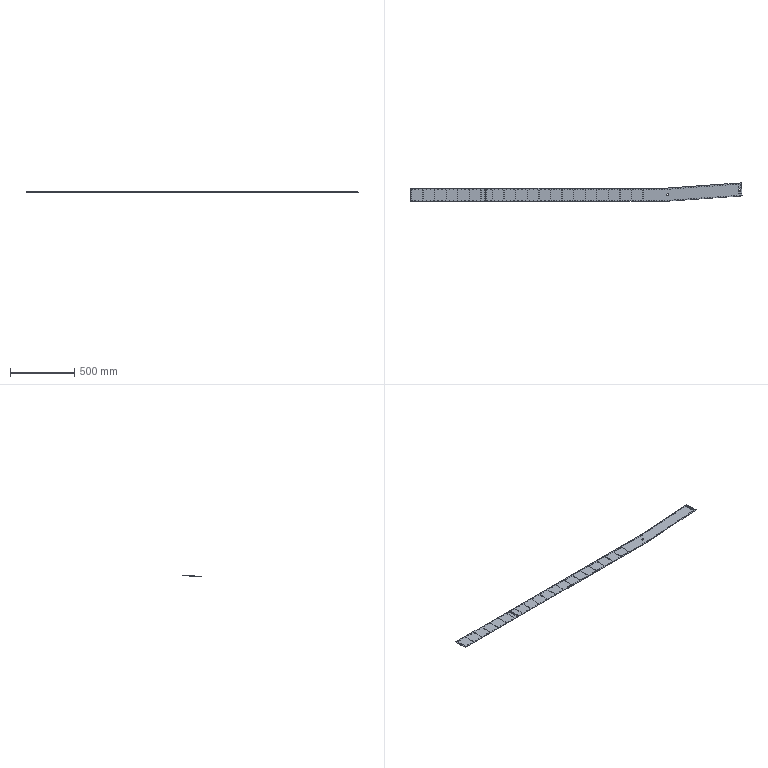Part | SolidWorks | features BaseBody 2 | 2 solids | 704 faces | box 2579 x 141.945 x 3.277 mm | volume 208042 mm3 | cylinder 690 | plane 14 | commonest cylinder face diameters 3.2 x456 2.4 x230 15.9 x4